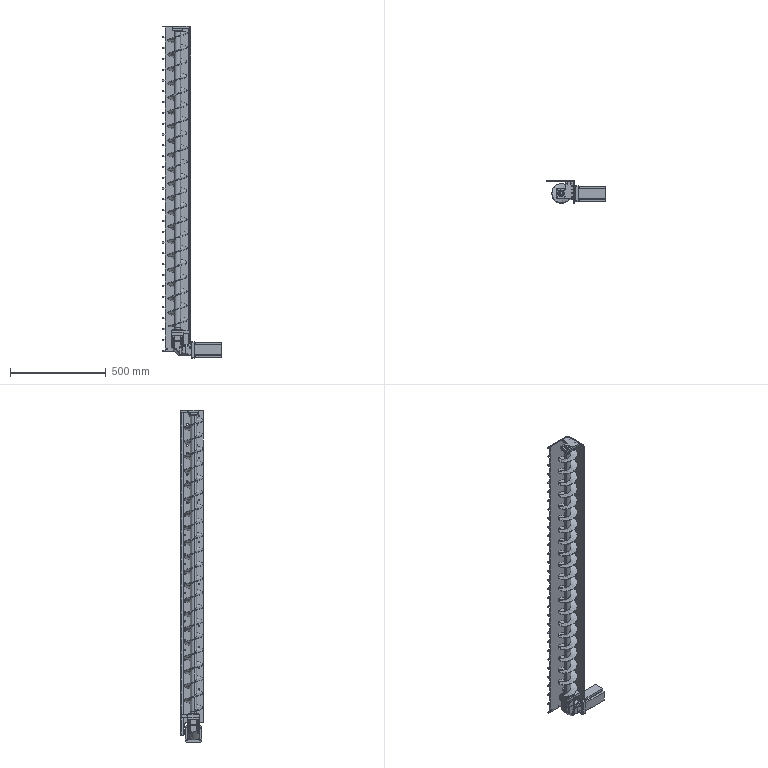Part | SolidWorks | features InContextFeatHolder 4 | 24 solids | 1247 faces | box 312 x 120 x 1735 mm | volume 4939212 mm3 | cylinder 582 | plane 463 | cone 125 | spline 53 | torus 24 | commonest cylinder face diameters 4.2 x94 6.8 x64 10 x52 5.8 x46 69 x26 3.3 x18